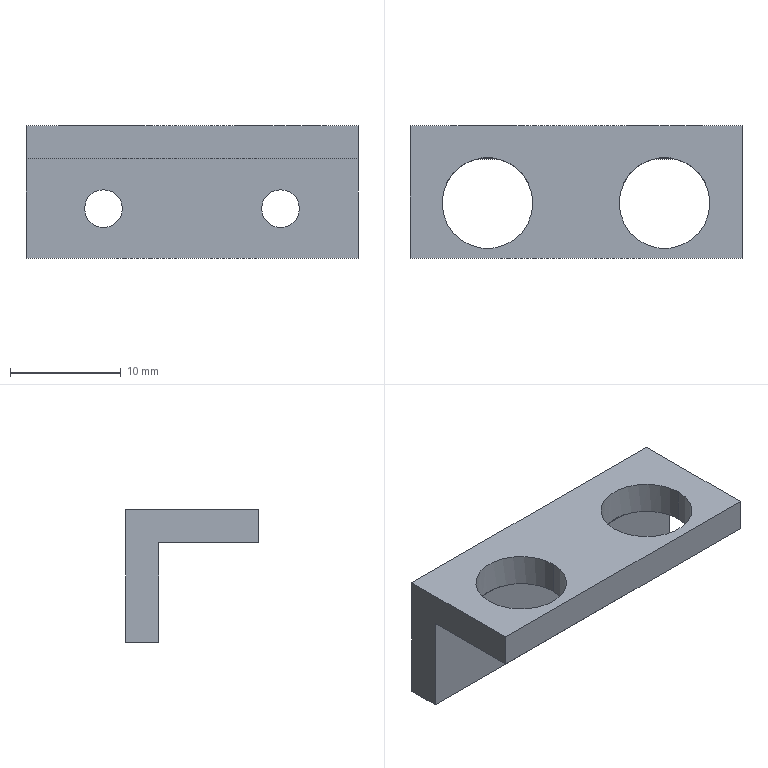NC program | NX | posted with a generic post | part box 30 x 12 x 12 mm
Whole program:
N10 G17 G21 G94 G90
(ZLEVEL_PROFILE , TOOL : D10)
N12 T04 M6
N14 G54
N16 G17 G0 G90 X17.552 Y-3.925 B0. C0. S3500 M3
N18 G43 Z30. H4
N20 Z-0.22
N22 G94 G1 X16.779 Y-2.594 F1000.
N24 G3 X15.912 Y-2.096 R1.
N26 G1 X14.354 Y-2.1 F2200.
N28 X-15.
N30 X-15.033 Y-2.097
N32 X-15.912 Y-2.096
N34 G3 X-16.778 Y-2.596 R1.
N36 G1 X-17.547 Y-3.926
N38 G0 X-17.549 Z-0.439
N40 G1 X-16.78 Y-2.596 F1000.
N42 G2 X-15.913 Y-2.096 R1.
N44 G1 X-15.033 Y-2.097 F2200.
N46 X-15. Y-2.1
N48 X14.354
N50 X15.913 Y-2.096
N52 G2 X16.781 Y-2.594 R1.
N54 G1 X17.553 Y-3.925
N56 G0 X17.554 Z-0.659
N58 G1 X16.782 Y-2.594 F1000.
N60 G3 X15.915 Y-2.096 R1.
N62 G1 X14.354 Y-2.1 F2200.
N64 X-15.
N66 X-15.033 Y-2.097
N68 X-15.915 Y-2.096
N70 G3 X-16.781 Y-2.596 R1.
N72 G1 X-17.55 Y-3.926
N74 G0 X-17.551 Z-0.878
N76 G1 X-16.782 Y-2.596 F1000.
N78 G2 X-15.916 Y-2.096 R1.
N80 G1 X-15. Y-2.1 F2200.
N82 X14.354
N84 X15.916 Y-2.096
N86 G2 X16.783 Y-2.594 R1.
N88 G1 X17.555 Y-3.924
N90 G0 X17.556 Z-1.098
N92 G1 X16.784 Y-2.594 F1000.
N94 G3 X15.917 Y-2.096 R1.
N96 G1 X14.354 Y-2.1 F2200.
N98 X-15.033 Y-2.097
N100 X-15.917 Y-2.096
N102 G3 X-16.783 Y-2.596 R1.
N104 G1 X-17.552 Y-3.926
N106 G0 X-17.554 Y-3.925 Z-1.317
N108 G1 X-16.785 Y-2.596 F1000.
N110 G2 X-15.918 Y-2.096 R1.
N112 G1 X-15. Y-2.1 F2200.
N114 X14.354
N116 X15.918 Y-2.096
N118 G2 X16.785 Y-2.594 R1.
N120 G1 X17.557 Y-3.924
N122 G0 X17.558 Z-1.537
N124 G1 X16.786 Y-2.595 F1000.
N126 G3 X15.919 Y-2.096 R1.
N128 G1 X14.354 Y-2.1 F2200.
N130 X-15.033 Y-2.097
N132 X-15.919 Y-2.096
N134 G3 X-16.786 Y-2.596 R1.
N136 G1 X-17.555 Y-3.925
N138 G0 X-17.556 Z-1.756
N140 G1 X-16.787 Y-2.596 F1000.
N142 G2 X-15.92 Y-2.097 R1.
N144 G1 X-15. Y-2.1 F2200.
N146 X14.354
N148 X15.92 Y-2.097
N150 G2 X16.788 Y-2.595 R1.
N152 G1 X17.559 Y-3.924
N154 G0 X17.56 Z-1.976
N156 G1 X16.789 Y-2.595 F1000.
N158 G3 X15.922 Y-2.097 R1.
N160 G1 X14.354 Y-2.1 F2200.
N162 X-15.033 Y-2.098
N164 X-15.922 Y-2.097
N166 G3 X-16.788 Y-2.596 R1.
N168 G1 X-17.557 Y-3.925
N170 G0 X-17.559 Y-3.924 Z-2.195
N172 G1 X-16.789 Y-2.596 F1000.
N174 G2 X-15.923 Y-2.097 R1.
N176 G1 X-15. Y-2.1 F2200.
N178 X14.354
N180 X15.923 Y-2.097
N182 G2 X16.79 Y-2.595 R1.
N184 G1 X17.561 Y-3.924
N186 G0 X17.562 Z-2.415
N188 G1 X16.791 Y-2.595 F1000.
N190 G3 X15.924 Y-2.097 R1.
N192 G1 X14.354 Y-2.1 F2200.
N194 X-15.033 Y-2.098
N196 X-15.924 Y-2.097
N198 G3 X-16.791 Y-2.596 R1.
N200 G1 X-17.56 Y-3.924
N202 G0 X-17.561 Z-2.634
N204 G1 X-16.792 Y-2.596 F1000.
N206 G2 X-15.925 Y-2.097 R1.
N208 G1 X-15. Y-2.1 F2200.
N210 X14.354
N212 X15.925 Y-2.097
N214 G2 X16.792 Y-2.595 R1.
N216 G1 X17.563 Y-3.923
N218 G0 X17.564 Z-2.854
N220 G1 X16.793 Y-2.595 F1000.
N222 G3 X15.926 Y-2.097 R1.
N224 G1 X14.354 Y-2.1 F2200.
N226 X-15.033 Y-2.098
N228 X-15.926 Y-2.097
N230 G3 X-16.793 Y-2.596 R1.
N232 G1 X-17.562 Y-3.924
N234 G0 X-17.569 Y-3.922 Z-3.073
N236 G1 X-16.795 Y-2.594 F1000.
N238 G2 X-15.928 Y-2.097 R1.
N240 G1 X-15. Y-2.1 F2200.
N242 X14.354
N244 X15.928 Y-2.097
N246 G2 X16.795 Y-2.595 R1.
N248 G1 X17.565 Y-3.923
N250 G0 X17.566 Z-3.293
N252 G1 X16.796 Y-2.595 F1000.
N254 G3 X15.929 Y-2.097 R1.
N256 G1 X14.354 Y-2.1 F2200.
N258 X-15.
N260 X-15.929 Y-2.097
N262 G3 X-16.796 Y-2.594 R1.
N264 G1 X-17.57 Y-3.922
N266 G0 Z-3.512
N268 G1 X-16.798 Y-2.594 F1000.
N270 G2 X-15.93 Y-2.097 R1.
N272 G1 X-15. Y-2.1 F2200.
N274 X14.354
N276 X15.93 Y-2.097
N278 G2 X16.797 Y-2.595 R1.
N280 G1 X17.567 Y-3.923
N282 G0 X17.568 Z-3.732
N284 G1 X16.798 Y-2.595 F1000.
N286 G3 X15.931 Y-2.097 R1.
N288 G1 X14.354 Y-2.1 F2200.
N290 X-15.
N292 X-15.931 Y-2.097
N294 G3 X-16.799 Y-2.594 R1.
N296 G1 X-17.571 Y-3.922
N298 G0 X-17.572 Z-3.951
N300 G1 X-16.8 Y-2.594 F1000.
N302 G2 X-15.932 Y-2.097 R1.
N304 G1 X-15. Y-2.1 F2200.
N306 X14.354
N308 X15.932 Y-2.097
N310 G2 X16.799 Y-2.595 R1.
N312 G1 X17.569 Y-3.922
N314 G0 X17.57 Z-4.171
N316 G1 X16.8 Y-2.595 F1000.
N318 G3 X15.933 Y-2.097 R1.
N320 G1 X14.354 Y-2.1 F2200.
N322 X-15.
N324 X-15.933 Y-2.097
N326 G3 X-16.801 Y-2.594 R1.
N328 G1 X-17.573 Y-3.922
N330 G0 X-17.574 Y-3.921 Z-4.39
N332 G1 X-16.802 Y-2.594 F1000.
N334 G2 X-15.935 Y-2.097 R1.
N336 G1 X-15. Y-2.1 F2200.
N338 X14.354
N340 X15.935 Y-2.097
N342 G2 X16.802 Y-2.595 R1.
N344 G1 X17.571 Y-3.922
N346 G0 X17.572 Z-4.61
N348 G1 X16.803 Y-2.595 F1000.
N350 G3 X15.936 Y-2.097 R1.
N352 G1 X14.354 Y-2.1 F2200.
N354 X-15.
N356 X-15.936 Y-2.097
N358 G3 X-16.803 Y-2.594 R1.
N360 G1 X-17.575 Y-3.921
N362 G0 X-17.576 Z-4.829
N364 G1 X-16.805 Y-2.594 F1000.
N366 G2 X-15.937 Y-2.097 R1.
N368 G1 X-15. Y-2.1 F2200.
N370 X14.354
N372 X15.937 Y-2.097
N374 G2 X16.804 Y-2.596 R1.
N376 G1 X17.573 Y-3.922
N378 G0 X17.574 Y-3.921 Z-5.049
N380 G1 X16.805 Y-2.596 F1000.
N382 G3 X15.938 Y-2.097 R1.
N384 G1 X14.354 Y-2.1 F2200.
N386 X-15.
N388 X-15.938 Y-2.097
N390 G3 X-16.806 Y-2.595 R1.
N392 G1 X-17.577 Y-3.921
N394 G0 X-17.718 Y-3.887 Z-5.268
N396 G1 X-16.833 Y-2.545 F1000.
N398 G2 X-15.939 Y-2.097 R1.
N400 G1 X-15. Y-2.1 F2200.
N402 X14.354
N404 X15.939 Y-2.097
N406 G2 X16.833 Y-2.545 R1.
N408 G1 X17.717 Y-3.887
N410 G0 X17.718 Z-5.488
N412 G1 X16.835 Y-2.545 F1000.
N414 G3 X15.941 Y-2.097 R1.
N416 G1 X14.354 Y-2.1 F2200.
N418 X-15.
N420 X-15.941 Y-2.097
N422 G3 X-16.835 Y-2.545 R1.
N424 G1 X-17.719 Y-3.887
N426 G0 X-17.72 Z-5.707
N428 G1 X-16.836 Y-2.545 F1000.
N430 G2 X-15.942 Y-2.097 R1.
N432 G1 X-15. Y-2.1 F2200.
N434 X14.354
N436 X15.942 Y-2.097
N438 G2 X16.836 Y-2.545 R1.
N440 G1 X17.719 Y-3.887
N442 G0 X17.72 Z-5.927
N444 G1 X16.837 Y-2.545 F1000.
N446 G3 X15.943 Y-2.097 R1.
N448 G1 X14.354 Y-2.1 F2200.
N450 X-15.
N452 X-15.943 Y-2.097
N454 G3 X-16.837 Y-2.545 R1.
N456 G1 X-17.721 Y-3.887
N458 G0 X-17.722 Z-6.146
N460 G1 X-16.838 Y-2.546 F1000.
N462 G2 X-15.944 Y-2.097 R1.
N464 G1 X-15. Y-2.1 F2200.
N466 X14.354
N468 X15.944 Y-2.097
N470 G2 X16.838 Y-2.546 R1.
N472 G1 X17.722 Y-3.887
N474 G0 X17.723 Y-3.886 Z-6.366
N476 G1 X16.839 Y-2.546 F1000.
N478 G3 X15.945 Y-2.097 R1.
N480 G1 X14.354 Y-2.1 F2200.
N482 X-15.
N484 X-15.945 Y-2.097
N486 G3 X-16.839 Y-2.546 R1.
N488 G1 X-17.723 Y-3.886
N490 G0 X-17.724 Z-6.585
N492 G1 X-16.84 Y-2.546 F1000.
N494 G2 X-15.947 Y-2.097 R1.
N496 G1 X-15. Y-2.1 F2200.
N498 X14.354
N500 X15.947 Y-2.097
N502 G2 X16.84 Y-2.546 R1.
N504 G1 X17.724 Y-3.886
N506 G0 X17.725 Z-6.805
N508 G1 X16.842 Y-2.546 F1000.
N510 G3 X15.948 Y-2.097 R1.
N512 G1 X14.354 Y-2.1 F2200.
N514 X-15.
N516 X-15.948 Y-2.097
N518 G3 X-16.842 Y-2.546 R1.
N520 G1 X-17.725 Y-3.886
N522 G0 X-17.726 Z-7.024
N524 G1 X-16.843 Y-2.546 F1000.
N526 G2 X-15.949 Y-2.098 R1.
N528 G1 X-15. Y-2.1 F2200.
N530 X14.354
N532 X15.949 Y-2.098
N534 G2 X16.843 Y-2.546 R1.
N536 G1 X17.726 Y-3.886
N538 G0 X17.727 Z-7.244
N540 G1 X16.844 Y-2.546 F1000.
N542 G3 X15.95 Y-2.098 R1.
N544 G1 X14.354 Y-2.1 F2200.
N546 X-15.
N548 X-15.95 Y-2.098
N550 G3 X-16.844 Y-2.546 R1.
N552 G1 X-17.727 Y-3.886
N554 G0 X-17.728 Y-3.885 Z-7.463
N556 G1 X-16.845 Y-2.546 F1000.
N558 G2 X-15.951 Y-2.098 R1.
N560 G1 X-15. Y-2.1 F2200.
N562 X14.354
N564 X15.951 Y-2.098
N566 G2 X16.845 Y-2.546 R1.
N568 G1 X17.728 Y-3.885
N570 G0 X17.729 Z-7.683
N572 G1 X16.846 Y-2.546 F1000.
N574 G3 X15.952 Y-2.098 R1.
N576 G1 X14.354 Y-2.1 F2200.
N578 X-15.
N580 X-15.952 Y-2.098
N582 G3 X-16.846 Y-2.546 R1.
N584 G1 X-17.729 Y-3.885
N586 G0 X-17.73 Z-7.902
N588 G1 X-16.848 Y-2.546 F1000.
N590 G2 X-15.954 Y-2.098 R1.
N592 G1 X-15. Y-2.1 F2200.
N594 X14.354
N596 X15.954 Y-2.098
N598 G2 X16.848 Y-2.546 R1.
N600 G1 X17.73 Y-3.885
N602 G0 X17.731 Z-8.122
N604 G1 X16.849 Y-2.546 F1000.
N606 G3 X15.955 Y-2.098 R1.
N608 G1 X14.354 Y-2.1 F2200.
N610 X-15.
N612 X-15.955 Y-2.098
N614 G3 X-16.849 Y-2.546 R1.
N616 G1 X-17.731 Y-3.885
N618 G0 X-17.732 Z-8.341
N620 G1 X-16.85 Y-2.546 F1000.
N622 G2 X-15.956 Y-2.098 R1.
N624 G1 X-15. Y-2.1 F2200.
N626 X14.354
N628 X15.956 Y-2.098
N630 G2 X16.85 Y-2.546 R1.
N632 G1 X17.732 Y-3.884
N634 G0 X17.733 Z-8.561
N636 G1 X16.851 Y-2.546 F1000.
N638 G3 X15.957 Y-2.098 R1.
N640 G1 X14.354 Y-2.1 F2200.
N642 X-15.
N644 X-15.957 Y-2.098
N646 G3 X-16.851 Y-2.546 R1.
N648 G1 X-17.733 Y-3.884
N650 G0 X-17.734 Z-8.78
N652 G1 X-16.852 Y-2.546 F1000.
N654 G2 X-15.958 Y-2.098 R1.
N656 G1 X-15. Y-2.1 F2200.
N658 X14.354
N660 X15.906 Y-2.101
N662 X15.958 Y-2.098
N664 G2 X16.852 Y-2.546 R1.
N666 G1 X17.734 Y-3.884
N668 G0 X17.735 Z-9.
N670 G1 X16.853 Y-2.546 F1000.
N672 G3 X15.96 Y-2.098 R1.
N674 G1 X15.906 Y-2.101 F2200.
N676 X14.354 Y-2.1
N678 X-15.
N680 X-15.906 Y-2.101
N682 X-15.96 Y-2.098
N684 G3 X-16.853 Y-2.546 R1.
N686 G1 X-17.735 Y-3.884
N688 G0 Z30.
N690 M5
(FLOOR_WALL_1_COPY_COPY , TOOL : D10JING)
N692 T14 M6
N694 G54
N696 G17 G0 G90 X21. Y-2. B0. C0. S7500 M3
N698 G43 Z30. H14
N700 Z-8.
N702 G94 G1 Z-9. F1000.
N704 X15.
N706 X-15. F1200.
N708 X-21.
N710 Z-8.
N712 G0 Z30.
N714 M5
(PLANAR_MILL_COPY_1_COPY_COPY_COPY , TOOL : D6A45)
N716 T01 M6
N718 G54
N720 G17 G0 G90 X0.766 Y1.743 B0. C0. S7500 M3
N722 G43 Z30. H1
N724 Z1.
N726 G94 G1 Z-1. F1250.
N728 G3 X0. Y2.1 R1.
N730 G1 X-15.
N732 G2 X-15.9 Y3. R0.9
N734 G1 Y6.
N736 G2 X-15. Y6.9 R0.9
N738 G1 X15.
N740 G2 X15.9 Y6. R0.9
N742 G1 Y3.
N744 G2 X15. Y2.1 R0.9
N746 G1 X0.
N748 G3 X-0.766 Y1.743 R1.
N750 G1 Z1.
N752 G0 Z30.
N754 M5
N756 M2